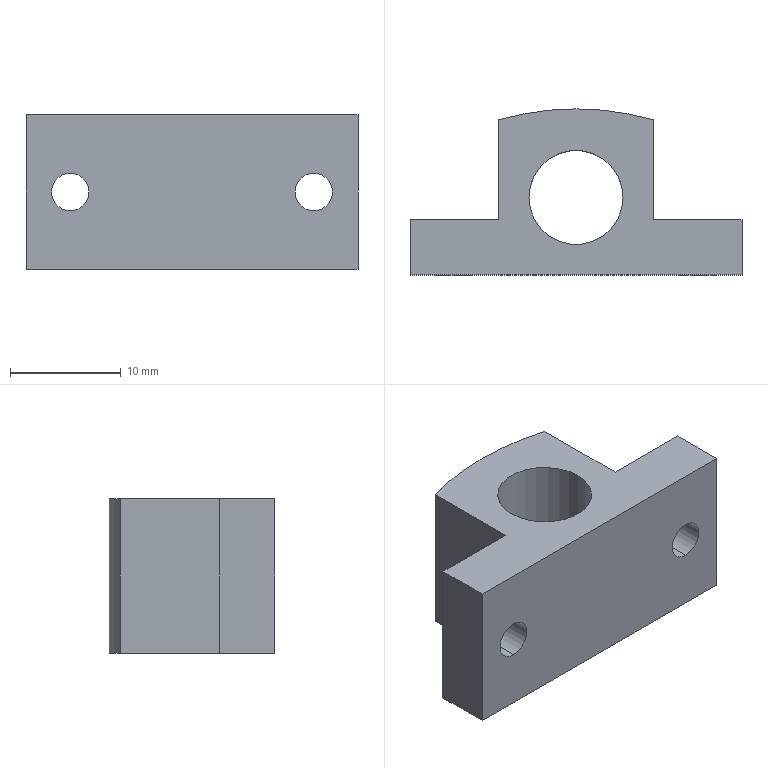Part | SolidWorks | features Extrusion 1, HoleWzd 1, ICE 1 | 1 solid | 20 faces | box 30 x 15 x 14 mm | volume 3079 mm3 | plane 9 | cylinder 7 | cone 4 | commonest cylinder face diameters 3.4 x4 8.5 x2 50 x1
STEP:
#1=CARTESIAN_POINT('',(-4.25,7.,-7.));
#2=VERTEX_POINT('',#1);
#3=CARTESIAN_POINT('',(4.25,7.,-7.));
#4=VERTEX_POINT('',#3);
#5=CARTESIAN_POINT('',(0.,7.,-7.));
#6=DIRECTION('',(0.,0.,1.));
#7=DIRECTION('',(1.,0.,0.));
#8=AXIS2_PLACEMENT_3D('',#5,#6,#7);
#9=CIRCLE('',#8,4.25);
#10=EDGE_CURVE('',#2,#4,#9,.T.);
#11=ORIENTED_EDGE('',*,*,#10,.F.);
#12=CARTESIAN_POINT('',(-4.25,7.,7.));
#13=VERTEX_POINT('',#12);
#14=CARTESIAN_POINT('',(-4.25,7.,-7.));
#15=DIRECTION('',(0.,0.,1.));
#16=VECTOR('',#15,1000.);
#17=LINE('',#14,#16);
#18=EDGE_CURVE('',#2,#13,#17,.T.);
#19=ORIENTED_EDGE('',*,*,#18,.T.);
#20=CARTESIAN_POINT('',(4.25,7.,7.));
#21=VERTEX_POINT('',#20);
#22=CARTESIAN_POINT('',(0.,7.,7.));
#23=DIRECTION('',(0.,0.,1.));
#24=DIRECTION('',(1.,0.,0.));
#25=AXIS2_PLACEMENT_3D('',#22,#23,#24);
#26=CIRCLE('',#25,4.25);
#27=EDGE_CURVE('',#13,#21,#26,.T.);
#28=ORIENTED_EDGE('',*,*,#27,.T.);
#29=CARTESIAN_POINT('',(4.25,7.,-7.));
#30=DIRECTION('',(0.,0.,1.));
#31=VECTOR('',#30,1000.);
#32=LINE('',#29,#31);
#33=EDGE_CURVE('',#4,#21,#32,.T.);
#34=ORIENTED_EDGE('',*,*,#33,.F.);
#35=EDGE_LOOP('',(#11,#19,#28,#34));
#36=FACE_OUTER_BOUND('',#35,.T.);
#37=CARTESIAN_POINT('',(0.,7.,-7.));
#38=DIRECTION('',(0.,0.,1.));
#39=DIRECTION('',(1.,0.,0.));
#40=AXIS2_PLACEMENT_3D('',#37,#38,#39);
#41=CYLINDRICAL_SURFACE('',#40,4.25);
#42=ADVANCED_FACE('',(#36),#41,.F.);
#43=CARTESIAN_POINT('',(-11.,3.5,-1.7));
#44=VERTEX_POINT('',#43);
#45=CARTESIAN_POINT('',(-11.,3.5,1.7));
#46=VERTEX_POINT('',#45);
#47=CARTESIAN_POINT('',(-11.,3.5,0.));
#48=DIRECTION('',(0.,1.,0.));
#49=DIRECTION('',(0.,0.,1.));
#50=AXIS2_PLACEMENT_3D('',#47,#48,#49);
#51=CIRCLE('',#50,1.7);
#52=EDGE_CURVE('',#44,#46,#51,.T.);
#53=ORIENTED_EDGE('',*,*,#52,.F.);
#54=CARTESIAN_POINT('',(-11.,5.,-3.2));
#55=VERTEX_POINT('',#54);
#56=CARTESIAN_POINT('',(-11.,5.,-3.2));
#57=DIRECTION('',(0.,0.7071,-0.7071));
#58=VECTOR('',#57,1000.);
#59=LINE('',#56,#58);
#60=EDGE_CURVE('',#44,#55,#59,.T.);
#61=ORIENTED_EDGE('',*,*,#60,.T.);
#62=CARTESIAN_POINT('',(-11.,5.,3.2));
#63=VERTEX_POINT('',#62);
#64=CARTESIAN_POINT('',(-11.,5.,0.));
#65=DIRECTION('',(0.,1.,0.));
#66=DIRECTION('',(0.,0.,1.));
#67=AXIS2_PLACEMENT_3D('',#64,#65,#66);
#68=CIRCLE('',#67,3.2);
#69=EDGE_CURVE('',#55,#63,#68,.T.);
#70=ORIENTED_EDGE('',*,*,#69,.T.);
#71=CARTESIAN_POINT('',(-11.,5.,3.2));
#72=DIRECTION('',(0.,0.7071,0.7071));
#73=VECTOR('',#72,1000.);
#74=LINE('',#71,#73);
#75=EDGE_CURVE('',#46,#63,#74,.T.);
#76=ORIENTED_EDGE('',*,*,#75,.F.);
#77=EDGE_LOOP('',(#53,#61,#70,#76));
#78=FACE_OUTER_BOUND('',#77,.T.);
#79=CARTESIAN_POINT('',(-11.,5.,0.));
#80=DIRECTION('',(0.,1.,0.));
#81=DIRECTION('',(0.,0.,1.));
#82=AXIS2_PLACEMENT_3D('',#79,#80,#81);
#83=CONICAL_SURFACE('',#82,3.2,0.7854);
#84=ADVANCED_FACE('',(#78),#83,.F.);
#85=CARTESIAN_POINT('',(-11.,0.,-1.7));
#86=VERTEX_POINT('',#85);
#87=CARTESIAN_POINT('',(-11.,0.,1.7));
#88=VERTEX_POINT('',#87);
#89=CARTESIAN_POINT('',(-11.,0.,0.));
#90=DIRECTION('',(0.,1.,0.));
#91=DIRECTION('',(0.,0.,1.));
#92=AXIS2_PLACEMENT_3D('',#89,#90,#91);
#93=CIRCLE('',#92,1.7);
#94=EDGE_CURVE('',#86,#88,#93,.T.);
#95=ORIENTED_EDGE('',*,*,#94,.F.);
#96=CARTESIAN_POINT('',(-11.,5.,-1.7));
#97=DIRECTION('',(0.,1.,0.));
#98=VECTOR('',#97,1000.);
#99=LINE('',#96,#98);
#100=EDGE_CURVE('',#86,#44,#99,.T.);
#101=ORIENTED_EDGE('',*,*,#100,.T.);
#102=ORIENTED_EDGE('',*,*,#52,.T.);
#103=CARTESIAN_POINT('',(-11.,5.,1.7));
#104=DIRECTION('',(0.,1.,0.));
#105=VECTOR('',#104,1000.);
#106=LINE('',#103,#105);
#107=EDGE_CURVE('',#88,#46,#106,.T.);
#108=ORIENTED_EDGE('',*,*,#107,.F.);
#109=EDGE_LOOP('',(#95,#101,#102,#108));
#110=FACE_OUTER_BOUND('',#109,.T.);
#111=CARTESIAN_POINT('',(-11.,5.,0.));
#112=DIRECTION('',(0.,1.,0.));
#113=DIRECTION('',(0.,0.,1.));
#114=AXIS2_PLACEMENT_3D('',#111,#112,#113);
#115=CYLINDRICAL_SURFACE('',#114,1.7);
#116=ADVANCED_FACE('',(#110),#115,.F.);
#117=CARTESIAN_POINT('',(11.,3.5,-1.7));
#118=VERTEX_POINT('',#117);
#119=CARTESIAN_POINT('',(11.,3.5,1.7));
#120=VERTEX_POINT('',#119);
#121=CARTESIAN_POINT('',(11.,3.5,0.));
#122=DIRECTION('',(0.,1.,0.));
#123=DIRECTION('',(0.,0.,1.));
#124=AXIS2_PLACEMENT_3D('',#121,#122,#123);
#125=CIRCLE('',#124,1.7);
#126=EDGE_CURVE('',#118,#120,#125,.T.);
#127=ORIENTED_EDGE('',*,*,#126,.F.);
#128=CARTESIAN_POINT('',(11.,5.,-3.2));
#129=VERTEX_POINT('',#128);
#130=CARTESIAN_POINT('',(11.,5.,-3.2));
#131=DIRECTION('',(0.,0.7071,-0.7071));
#132=VECTOR('',#131,1000.);
#133=LINE('',#130,#132);
#134=EDGE_CURVE('',#118,#129,#133,.T.);
#135=ORIENTED_EDGE('',*,*,#134,.T.);
#136=CARTESIAN_POINT('',(11.,5.,3.2));
#137=VERTEX_POINT('',#136);
#138=CARTESIAN_POINT('',(11.,5.,0.));
#139=DIRECTION('',(0.,1.,0.));
#140=DIRECTION('',(0.,0.,1.));
#141=AXIS2_PLACEMENT_3D('',#138,#139,#140);
#142=CIRCLE('',#141,3.2);
#143=EDGE_CURVE('',#129,#137,#142,.T.);
#144=ORIENTED_EDGE('',*,*,#143,.T.);
#145=CARTESIAN_POINT('',(11.,5.,3.2));
#146=DIRECTION('',(0.,0.7071,0.7071));
#147=VECTOR('',#146,1000.);
#148=LINE('',#145,#147);
#149=EDGE_CURVE('',#120,#137,#148,.T.);
#150=ORIENTED_EDGE('',*,*,#149,.F.);
#151=EDGE_LOOP('',(#127,#135,#144,#150));
#152=FACE_OUTER_BOUND('',#151,.T.);
#153=CARTESIAN_POINT('',(11.,5.,0.));
#154=DIRECTION('',(0.,1.,0.));
#155=DIRECTION('',(0.,0.,1.));
#156=AXIS2_PLACEMENT_3D('',#153,#154,#155);
#157=CONICAL_SURFACE('',#156,3.2,0.7854);
#158=ADVANCED_FACE('',(#152),#157,.F.);
#159=CARTESIAN_POINT('',(11.,0.,-1.7));
#160=VERTEX_POINT('',#159);
#161=CARTESIAN_POINT('',(11.,0.,1.7));
#162=VERTEX_POINT('',#161);
#163=CARTESIAN_POINT('',(11.,0.,0.));
#164=DIRECTION('',(0.,1.,0.));
#165=DIRECTION('',(0.,0.,1.));
#166=AXIS2_PLACEMENT_3D('',#163,#164,#165);
#167=CIRCLE('',#166,1.7);
#168=EDGE_CURVE('',#160,#162,#167,.T.);
#169=ORIENTED_EDGE('',*,*,#168,.F.);
#170=CARTESIAN_POINT('',(11.,5.,-1.7));
#171=DIRECTION('',(0.,1.,0.));
#172=VECTOR('',#171,1000.);
#173=LINE('',#170,#172);
#174=EDGE_CURVE('',#160,#118,#173,.T.);
#175=ORIENTED_EDGE('',*,*,#174,.T.);
#176=ORIENTED_EDGE('',*,*,#126,.T.);
#177=CARTESIAN_POINT('',(11.,5.,1.7));
#178=DIRECTION('',(0.,1.,0.));
#179=VECTOR('',#178,1000.);
#180=LINE('',#177,#179);
#181=EDGE_CURVE('',#162,#120,#180,.T.);
#182=ORIENTED_EDGE('',*,*,#181,.F.);
#183=EDGE_LOOP('',(#169,#175,#176,#182));
#184=FACE_OUTER_BOUND('',#183,.T.);
#185=CARTESIAN_POINT('',(11.,5.,0.));
#186=DIRECTION('',(0.,1.,0.));
#187=DIRECTION('',(0.,0.,1.));
#188=AXIS2_PLACEMENT_3D('',#185,#186,#187);
#189=CYLINDRICAL_SURFACE('',#188,1.7);
#190=ADVANCED_FACE('',(#184),#189,.F.);
#191=CARTESIAN_POINT('',(15.,0.,-7.));
#192=VERTEX_POINT('',#191);
#193=CARTESIAN_POINT('',(15.,5.,-7.));
#194=VERTEX_POINT('',#193);
#195=CARTESIAN_POINT('',(15.,5.,-7.));
#196=DIRECTION('',(0.,1.,0.));
#197=VECTOR('',#196,1000.);
#198=LINE('',#195,#197);
#199=EDGE_CURVE('',#192,#194,#198,.T.);
#200=ORIENTED_EDGE('',*,*,#199,.T.);
#201=CARTESIAN_POINT('',(15.,5.,7.));
#202=VERTEX_POINT('',#201);
#203=CARTESIAN_POINT('',(15.,5.,7.));
#204=DIRECTION('',(0.,0.,-1.));
#205=VECTOR('',#204,1000.);
#206=LINE('',#203,#205);
#207=EDGE_CURVE('',#202,#194,#206,.T.);
#208=ORIENTED_EDGE('',*,*,#207,.F.);
#209=CARTESIAN_POINT('',(15.,0.,7.));
#210=VERTEX_POINT('',#209);
#211=CARTESIAN_POINT('',(15.,5.,7.));
#212=DIRECTION('',(0.,1.,0.));
#213=VECTOR('',#212,1000.);
#214=LINE('',#211,#213);
#215=EDGE_CURVE('',#210,#202,#214,.T.);
#216=ORIENTED_EDGE('',*,*,#215,.F.);
#217=CARTESIAN_POINT('',(15.,0.,7.));
#218=DIRECTION('',(0.,0.,-1.));
#219=VECTOR('',#218,1000.);
#220=LINE('',#217,#219);
#221=EDGE_CURVE('',#210,#192,#220,.T.);
#222=ORIENTED_EDGE('',*,*,#221,.T.);
#223=EDGE_LOOP('',(#200,#208,#216,#222));
#224=FACE_OUTER_BOUND('',#223,.T.);
#225=CARTESIAN_POINT('',(15.,5.,7.));
#226=DIRECTION('',(-1.,0.,0.));
#227=DIRECTION('',(0.,-1.,0.));
#228=AXIS2_PLACEMENT_3D('',#225,#226,#227);
#229=PLANE('',#228);
#230=ADVANCED_FACE('',(#224),#229,.F.);
#231=CARTESIAN_POINT('',(11.,5.,0.));
#232=DIRECTION('',(0.,1.,0.));
#233=DIRECTION('',(0.,0.,1.));
#234=AXIS2_PLACEMENT_3D('',#231,#232,#233);
#235=CIRCLE('',#234,3.2);
#236=EDGE_CURVE('',#137,#129,#235,.T.);
#237=ORIENTED_EDGE('',*,*,#236,.F.);
#238=ORIENTED_EDGE('',*,*,#143,.F.);
#239=EDGE_LOOP('',(#237,#238));
#240=FACE_BOUND('',#239,.T.);
#241=CARTESIAN_POINT('',(7.,5.,-7.));
#242=VERTEX_POINT('',#241);
#243=CARTESIAN_POINT('',(15.,5.,-7.));
#244=DIRECTION('',(-1.,0.,0.));
#245=VECTOR('',#244,1000.);
#246=LINE('',#243,#245);
#247=EDGE_CURVE('',#194,#242,#246,.T.);
#248=ORIENTED_EDGE('',*,*,#247,.T.);
#249=CARTESIAN_POINT('',(7.,5.,7.));
#250=VERTEX_POINT('',#249);
#251=CARTESIAN_POINT('',(7.,5.,7.));
#252=DIRECTION('',(0.,0.,-1.));
#253=VECTOR('',#252,1000.);
#254=LINE('',#251,#253);
#255=EDGE_CURVE('',#250,#242,#254,.T.);
#256=ORIENTED_EDGE('',*,*,#255,.F.);
#257=CARTESIAN_POINT('',(15.,5.,7.));
#258=DIRECTION('',(-1.,0.,0.));
#259=VECTOR('',#258,1000.);
#260=LINE('',#257,#259);
#261=EDGE_CURVE('',#202,#250,#260,.T.);
#262=ORIENTED_EDGE('',*,*,#261,.F.);
#263=ORIENTED_EDGE('',*,*,#207,.T.);
#264=EDGE_LOOP('',(#248,#256,#262,#263));
#265=FACE_OUTER_BOUND('',#264,.T.);
#266=CARTESIAN_POINT('',(15.,5.,7.));
#267=DIRECTION('',(0.,-1.,0.));
#268=DIRECTION('',(1.,0.,0.));
#269=AXIS2_PLACEMENT_3D('',#266,#267,#268);
#270=PLANE('',#269);
#271=ADVANCED_FACE('',(#240,#265),#270,.F.);
#272=CARTESIAN_POINT('',(7.,14.,-7.));
#273=VERTEX_POINT('',#272);
#274=CARTESIAN_POINT('',(7.,5.,-7.));
#275=DIRECTION('',(0.,1.,0.));
#276=VECTOR('',#275,1000.);
#277=LINE('',#274,#276);
#278=EDGE_CURVE('',#242,#273,#277,.T.);
#279=ORIENTED_EDGE('',*,*,#278,.T.);
#280=CARTESIAN_POINT('',(7.,14.,7.));
#281=VERTEX_POINT('',#280);
#282=CARTESIAN_POINT('',(7.,14.,7.));
#283=DIRECTION('',(0.,0.,-1.));
#284=VECTOR('',#283,1000.);
#285=LINE('',#282,#284);
#286=EDGE_CURVE('',#281,#273,#285,.T.);
#287=ORIENTED_EDGE('',*,*,#286,.F.);
#288=CARTESIAN_POINT('',(7.,5.,7.));
#289=DIRECTION('',(0.,1.,0.));
#290=VECTOR('',#289,1000.);
#291=LINE('',#288,#290);
#292=EDGE_CURVE('',#250,#281,#291,.T.);
#293=ORIENTED_EDGE('',*,*,#292,.F.);
#294=ORIENTED_EDGE('',*,*,#255,.T.);
#295=EDGE_LOOP('',(#279,#287,#293,#294));
#296=FACE_OUTER_BOUND('',#295,.T.);
#297=CARTESIAN_POINT('',(7.,5.,7.));
#298=DIRECTION('',(-1.,0.,0.));
#299=DIRECTION('',(0.,-1.,0.));
#300=AXIS2_PLACEMENT_3D('',#297,#298,#299);
#301=PLANE('',#300);
#302=ADVANCED_FACE('',(#296),#301,.F.);
#303=CARTESIAN_POINT('',(-7.,14.,-7.));
#304=VERTEX_POINT('',#303);
#305=CARTESIAN_POINT('',(0.,-10.,-7.));
#306=DIRECTION('',(0.,0.,1.));
#307=DIRECTION('',(-1.,0.,0.));
#308=AXIS2_PLACEMENT_3D('',#305,#306,#307);
#309=CIRCLE('',#308,25.);
#310=EDGE_CURVE('',#273,#304,#309,.T.);
#311=ORIENTED_EDGE('',*,*,#310,.T.);
#312=CARTESIAN_POINT('',(-7.,14.,7.));
#313=VERTEX_POINT('',#312);
#314=CARTESIAN_POINT('',(-7.,14.,7.));
#315=DIRECTION('',(0.,0.,-1.));
#316=VECTOR('',#315,1000.);
#317=LINE('',#314,#316);
#318=EDGE_CURVE('',#313,#304,#317,.T.);
#319=ORIENTED_EDGE('',*,*,#318,.F.);
#320=CARTESIAN_POINT('',(0.,-10.,7.));
#321=DIRECTION('',(0.,0.,1.));
#322=DIRECTION('',(-1.,0.,0.));
#323=AXIS2_PLACEMENT_3D('',#320,#321,#322);
#324=CIRCLE('',#323,25.);
#325=EDGE_CURVE('',#281,#313,#324,.T.);
#326=ORIENTED_EDGE('',*,*,#325,.F.);
#327=ORIENTED_EDGE('',*,*,#286,.T.);
#328=EDGE_LOOP('',(#311,#319,#326,#327));
#329=FACE_OUTER_BOUND('',#328,.T.);
#330=CARTESIAN_POINT('',(0.,-10.,7.));
#331=DIRECTION('',(0.,0.,-1.));
#332=DIRECTION('',(-1.,0.,0.));
#333=AXIS2_PLACEMENT_3D('',#330,#331,#332);
#334=CYLINDRICAL_SURFACE('',#333,25.);
#335=ADVANCED_FACE('',(#329),#334,.T.);
#336=CARTESIAN_POINT('',(-7.,5.,-7.));
#337=VERTEX_POINT('',#336);
#338=CARTESIAN_POINT('',(-7.,5.,-7.));
#339=DIRECTION('',(0.,-1.,0.));
#340=VECTOR('',#339,1000.);
#341=LINE('',#338,#340);
#342=EDGE_CURVE('',#304,#337,#341,.T.);
#343=ORIENTED_EDGE('',*,*,#342,.T.);
#344=CARTESIAN_POINT('',(-7.,5.,7.));
#345=VERTEX_POINT('',#344);
#346=CARTESIAN_POINT('',(-7.,5.,7.));
#347=DIRECTION('',(0.,0.,-1.));
#348=VECTOR('',#347,1000.);
#349=LINE('',#346,#348);
#350=EDGE_CURVE('',#345,#337,#349,.T.);
#351=ORIENTED_EDGE('',*,*,#350,.F.);
#352=CARTESIAN_POINT('',(-7.,5.,7.));
#353=DIRECTION('',(0.,-1.,0.));
#354=VECTOR('',#353,1000.);
#355=LINE('',#352,#354);
#356=EDGE_CURVE('',#313,#345,#355,.T.);
#357=ORIENTED_EDGE('',*,*,#356,.F.);
#358=ORIENTED_EDGE('',*,*,#318,.T.);
#359=EDGE_LOOP('',(#343,#351,#357,#358));
#360=FACE_OUTER_BOUND('',#359,.T.);
#361=CARTESIAN_POINT('',(-7.,5.,7.));
#362=DIRECTION('',(1.,0.,0.));
#363=DIRECTION('',(0.,0.,-1.));
#364=AXIS2_PLACEMENT_3D('',#361,#362,#363);
#365=PLANE('',#364);
#366=ADVANCED_FACE('',(#360),#365,.F.);
#367=CARTESIAN_POINT('',(-11.,5.,0.));
#368=DIRECTION('',(0.,1.,0.));
#369=DIRECTION('',(0.,0.,1.));
#370=AXIS2_PLACEMENT_3D('',#367,#368,#369);
#371=CIRCLE('',#370,3.2);
#372=EDGE_CURVE('',#63,#55,#371,.T.);
#373=ORIENTED_EDGE('',*,*,#372,.F.);
#374=ORIENTED_EDGE('',*,*,#69,.F.);
#375=EDGE_LOOP('',(#373,#374));
#376=FACE_BOUND('',#375,.T.);
#377=CARTESIAN_POINT('',(-15.,5.,-7.));
#378=VERTEX_POINT('',#377);
#379=CARTESIAN_POINT('',(-15.,5.,-7.));
#380=DIRECTION('',(-1.,0.,0.));
#381=VECTOR('',#380,1000.);
#382=LINE('',#379,#381);
#383=EDGE_CURVE('',#337,#378,#382,.T.);
#384=ORIENTED_EDGE('',*,*,#383,.T.);
#385=CARTESIAN_POINT('',(-15.,5.,7.));
#386=VERTEX_POINT('',#385);
#387=CARTESIAN_POINT('',(-15.,5.,7.));
#388=DIRECTION('',(0.,0.,-1.));
#389=VECTOR('',#388,1000.);
#390=LINE('',#387,#389);
#391=EDGE_CURVE('',#386,#378,#390,.T.);
#392=ORIENTED_EDGE('',*,*,#391,.F.);
#393=CARTESIAN_POINT('',(-15.,5.,7.));
#394=DIRECTION('',(-1.,0.,0.));
#395=VECTOR('',#394,1000.);
#396=LINE('',#393,#395);
#397=EDGE_CURVE('',#345,#386,#396,.T.);
#398=ORIENTED_EDGE('',*,*,#397,.F.);
#399=ORIENTED_EDGE('',*,*,#350,.T.);
#400=EDGE_LOOP('',(#384,#392,#398,#399));
#401=FACE_OUTER_BOUND('',#400,.T.);
#402=CARTESIAN_POINT('',(-15.,5.,7.));
#403=DIRECTION('',(0.,-1.,0.));
#404=DIRECTION('',(0.,0.,-1.));
#405=AXIS2_PLACEMENT_3D('',#402,#403,#404);
#406=PLANE('',#405);
#407=ADVANCED_FACE('',(#376,#401),#406,.F.);
#408=CARTESIAN_POINT('',(-15.,0.,-7.));
#409=VERTEX_POINT('',#408);
#410=CARTESIAN_POINT('',(-15.,5.,-7.));
#411=DIRECTION('',(0.,-1.,0.));
#412=VECTOR('',#411,1000.);
#413=LINE('',#410,#412);
#414=EDGE_CURVE('',#378,#409,#413,.T.);
#415=ORIENTED_EDGE('',*,*,#414,.T.);
#416=CARTESIAN_POINT('',(-15.,0.,7.));
#417=VERTEX_POINT('',#416);
#418=CARTESIAN_POINT('',(-15.,0.,7.));
#419=DIRECTION('',(0.,0.,-1.));
#420=VECTOR('',#419,1000.);
#421=LINE('',#418,#420);
#422=EDGE_CURVE('',#417,#409,#421,.T.);
#423=ORIENTED_EDGE('',*,*,#422,.F.);
#424=CARTESIAN_POINT('',(-15.,5.,7.));
#425=DIRECTION('',(0.,-1.,0.));
#426=VECTOR('',#425,1000.);
#427=LINE('',#424,#426);
#428=EDGE_CURVE('',#386,#417,#427,.T.);
#429=ORIENTED_EDGE('',*,*,#428,.F.);
#430=ORIENTED_EDGE('',*,*,#391,.T.);
#431=EDGE_LOOP('',(#415,#423,#429,#430));
#432=FACE_OUTER_BOUND('',#431,.T.);
#433=CARTESIAN_POINT('',(-15.,5.,7.));
#434=DIRECTION('',(1.,0.,0.));
#435=DIRECTION('',(0.,0.,-1.));
#436=AXIS2_PLACEMENT_3D('',#433,#434,#435);
#437=PLANE('',#436);
#438=ADVANCED_FACE('',(#432),#437,.F.);
#439=CARTESIAN_POINT('',(-11.,0.,0.));
#440=DIRECTION('',(0.,1.,0.));
#441=DIRECTION('',(0.,0.,1.));
#442=AXIS2_PLACEMENT_3D('',#439,#440,#441);
#443=CIRCLE('',#442,1.7);
#444=EDGE_CURVE('',#88,#86,#443,.T.);
#445=ORIENTED_EDGE('',*,*,#444,.T.);
#446=ORIENTED_EDGE('',*,*,#94,.T.);
#447=EDGE_LOOP('',(#445,#446));
#448=FACE_BOUND('',#447,.T.);
#449=CARTESIAN_POINT('',(11.,0.,0.));
#450=DIRECTION('',(0.,1.,0.));
#451=DIRECTION('',(0.,0.,1.));
#452=AXIS2_PLACEMENT_3D('',#449,#450,#451);
#453=CIRCLE('',#452,1.7);
#454=EDGE_CURVE('',#162,#160,#453,.T.);
#455=ORIENTED_EDGE('',*,*,#454,.T.);
#456=ORIENTED_EDGE('',*,*,#168,.T.);
#457=EDGE_LOOP('',(#455,#456));
#458=FACE_BOUND('',#457,.T.);
#459=CARTESIAN_POINT('',(-15.,0.,-7.));
#460=DIRECTION('',(1.,0.,0.));
#461=VECTOR('',#460,1000.);
#462=LINE('',#459,#461);
#463=EDGE_CURVE('',#409,#192,#462,.T.);
#464=ORIENTED_EDGE('',*,*,#463,.T.);
#465=ORIENTED_EDGE('',*,*,#221,.F.);
#466=CARTESIAN_POINT('',(-15.,0.,7.));
#467=DIRECTION('',(1.,0.,0.));
#468=VECTOR('',#467,1000.);
#469=LINE('',#466,#468);
#470=EDGE_CURVE('',#417,#210,#469,.T.);
#471=ORIENTED_EDGE('',*,*,#470,.F.);
#472=ORIENTED_EDGE('',*,*,#422,.T.);
#473=EDGE_LOOP('',(#464,#465,#471,#472));
#474=FACE_OUTER_BOUND('',#473,.T.);
#475=CARTESIAN_POINT('',(-15.,0.,7.));
#476=DIRECTION('',(0.,1.,0.));
#477=DIRECTION('',(-1.,0.,0.));
#478=AXIS2_PLACEMENT_3D('',#475,#476,#477);
#479=PLANE('',#478);
#480=ADVANCED_FACE('',(#448,#458,#474),#479,.F.);
#481=CARTESIAN_POINT('',(0.,7.,7.));
#482=DIRECTION('',(0.,0.,1.));
#483=DIRECTION('',(1.,0.,0.));
#484=AXIS2_PLACEMENT_3D('',#481,#482,#483);
#485=CIRCLE('',#484,4.25);
#486=EDGE_CURVE('',#21,#13,#485,.T.);
#487=ORIENTED_EDGE('',*,*,#486,.F.);
#488=ORIENTED_EDGE('',*,*,#27,.F.);
#489=EDGE_LOOP('',(#487,#488));
#490=FACE_BOUND('',#489,.T.);
#491=ORIENTED_EDGE('',*,*,#215,.T.);
#492=ORIENTED_EDGE('',*,*,#261,.T.);
#493=ORIENTED_EDGE('',*,*,#292,.T.);
#494=ORIENTED_EDGE('',*,*,#325,.T.);
#495=ORIENTED_EDGE('',*,*,#356,.T.);
#496=ORIENTED_EDGE('',*,*,#397,.T.);
#497=ORIENTED_EDGE('',*,*,#428,.T.);
#498=ORIENTED_EDGE('',*,*,#470,.T.);
#499=EDGE_LOOP('',(#491,#492,#493,#494,#495,#496,#497,#498));
#500=FACE_OUTER_BOUND('',#499,.T.);
#501=CARTESIAN_POINT('',(0.,-10.,7.));
#502=DIRECTION('',(0.,0.,-1.));
#503=DIRECTION('',(-1.,0.,0.));
#504=AXIS2_PLACEMENT_3D('',#501,#502,#503);
#505=PLANE('',#504);
#506=ADVANCED_FACE('',(#490,#500),#505,.F.);
#507=CARTESIAN_POINT('',(0.,7.,-7.));
#508=DIRECTION('',(0.,0.,1.));
#509=DIRECTION('',(1.,0.,0.));
#510=AXIS2_PLACEMENT_3D('',#507,#508,#509);
#511=CIRCLE('',#510,4.25);
#512=EDGE_CURVE('',#4,#2,#511,.T.);
#513=ORIENTED_EDGE('',*,*,#512,.T.);
#514=ORIENTED_EDGE('',*,*,#10,.T.);
#515=EDGE_LOOP('',(#513,#514));
#516=FACE_BOUND('',#515,.T.);
#517=ORIENTED_EDGE('',*,*,#199,.F.);
#518=ORIENTED_EDGE('',*,*,#463,.F.);
#519=ORIENTED_EDGE('',*,*,#414,.F.);
#520=ORIENTED_EDGE('',*,*,#383,.F.);
#521=ORIENTED_EDGE('',*,*,#342,.F.);
#522=ORIENTED_EDGE('',*,*,#310,.F.);
#523=ORIENTED_EDGE('',*,*,#278,.F.);
#524=ORIENTED_EDGE('',*,*,#247,.F.);
#525=EDGE_LOOP('',(#517,#518,#519,#520,#521,#522,#523,#524));
#526=FACE_OUTER_BOUND('',#525,.T.);
#527=CARTESIAN_POINT('',(0.,-10.,-7.));
#528=DIRECTION('',(0.,0.,-1.));
#529=DIRECTION('',(-1.,0.,0.));
#530=AXIS2_PLACEMENT_3D('',#527,#528,#529);
#531=PLANE('',#530);
#532=ADVANCED_FACE('',(#516,#526),#531,.T.);
#533=ORIENTED_EDGE('',*,*,#174,.F.);
#534=ORIENTED_EDGE('',*,*,#454,.F.);
#535=ORIENTED_EDGE('',*,*,#181,.T.);
#536=CARTESIAN_POINT('',(11.,3.5,0.));
#537=DIRECTION('',(0.,1.,0.));
#538=DIRECTION('',(0.,0.,1.));
#539=AXIS2_PLACEMENT_3D('',#536,#537,#538);
#540=CIRCLE('',#539,1.7);
#541=EDGE_CURVE('',#120,#118,#540,.T.);
#542=ORIENTED_EDGE('',*,*,#541,.T.);
#543=EDGE_LOOP('',(#533,#534,#535,#542));
#544=FACE_OUTER_BOUND('',#543,.T.);
#545=CARTESIAN_POINT('',(11.,5.,0.));
#546=DIRECTION('',(0.,1.,0.));
#547=DIRECTION('',(0.,0.,1.));
#548=AXIS2_PLACEMENT_3D('',#545,#546,#547);
#549=CYLINDRICAL_SURFACE('',#548,1.7);
#550=ADVANCED_FACE('',(#544),#549,.F.);
#551=ORIENTED_EDGE('',*,*,#134,.F.);
#552=ORIENTED_EDGE('',*,*,#541,.F.);
#553=ORIENTED_EDGE('',*,*,#149,.T.);
#554=ORIENTED_EDGE('',*,*,#236,.T.);
#555=EDGE_LOOP('',(#551,#552,#553,#554));
#556=FACE_OUTER_BOUND('',#555,.T.);
#557=CARTESIAN_POINT('',(11.,5.,0.));
#558=DIRECTION('',(0.,1.,0.));
#559=DIRECTION('',(0.,0.,1.));
#560=AXIS2_PLACEMENT_3D('',#557,#558,#559);
#561=CONICAL_SURFACE('',#560,3.2,0.7854);
#562=ADVANCED_FACE('',(#556),#561,.F.);
#563=ORIENTED_EDGE('',*,*,#100,.F.);
#564=ORIENTED_EDGE('',*,*,#444,.F.);
#565=ORIENTED_EDGE('',*,*,#107,.T.);
#566=CARTESIAN_POINT('',(-11.,3.5,0.));
#567=DIRECTION('',(0.,1.,0.));
#568=DIRECTION('',(0.,0.,1.));
#569=AXIS2_PLACEMENT_3D('',#566,#567,#568);
#570=CIRCLE('',#569,1.7);
#571=EDGE_CURVE('',#46,#44,#570,.T.);
#572=ORIENTED_EDGE('',*,*,#571,.T.);
#573=EDGE_LOOP('',(#563,#564,#565,#572));
#574=FACE_OUTER_BOUND('',#573,.T.);
#575=CARTESIAN_POINT('',(-11.,5.,0.));
#576=DIRECTION('',(0.,1.,0.));
#577=DIRECTION('',(0.,0.,1.));
#578=AXIS2_PLACEMENT_3D('',#575,#576,#577);
#579=CYLINDRICAL_SURFACE('',#578,1.7);
#580=ADVANCED_FACE('',(#574),#579,.F.);
#581=ORIENTED_EDGE('',*,*,#60,.F.);
#582=ORIENTED_EDGE('',*,*,#571,.F.);
#583=ORIENTED_EDGE('',*,*,#75,.T.);
#584=ORIENTED_EDGE('',*,*,#372,.T.);
#585=EDGE_LOOP('',(#581,#582,#583,#584));
#586=FACE_OUTER_BOUND('',#585,.T.);
#587=CARTESIAN_POINT('',(-11.,5.,0.));
#588=DIRECTION('',(0.,1.,0.));
#589=DIRECTION('',(0.,0.,1.));
#590=AXIS2_PLACEMENT_3D('',#587,#588,#589);
#591=CONICAL_SURFACE('',#590,3.2,0.7854);
#592=ADVANCED_FACE('',(#586),#591,.F.);
#593=ORIENTED_EDGE('',*,*,#18,.F.);
#594=ORIENTED_EDGE('',*,*,#512,.F.);
#595=ORIENTED_EDGE('',*,*,#33,.T.);
#596=ORIENTED_EDGE('',*,*,#486,.T.);
#597=EDGE_LOOP('',(#593,#594,#595,#596));
#598=FACE_OUTER_BOUND('',#597,.T.);
#599=CARTESIAN_POINT('',(0.,7.,-7.));
#600=DIRECTION('',(0.,0.,1.));
#601=DIRECTION('',(1.,0.,0.));
#602=AXIS2_PLACEMENT_3D('',#599,#600,#601);
#603=CYLINDRICAL_SURFACE('',#602,4.25);
#604=ADVANCED_FACE('',(#598),#603,.F.);
#605=CLOSED_SHELL('',(#42,#84,#116,#158,#190,#230,#271,#302,#335,#366,#407,#438,#480,#506,#532,#550,#562,#580,#592,#604));
#606=MANIFOLD_SOLID_BREP('',#605);
#607=CARTESIAN_POINT('',(0.,0.,0.));
#608=DIRECTION('',(0.,0.,1.));
#609=DIRECTION('',(1.,0.,0.));
#610=AXIS2_PLACEMENT_3D('',#607,#608,#609);
#611=(LENGTH_UNIT()NAMED_UNIT(*)SI_UNIT(.MILLI.,.METRE.));
#612=UNCERTAINTY_MEASURE_WITH_UNIT(LENGTH_MEASURE(0.00001),#611,'','');
#613=(NAMED_UNIT(*)PLANE_ANGLE_UNIT()SI_UNIT($,.RADIAN.));
#614=(NAMED_UNIT(*)SI_UNIT($,.STERADIAN.)SOLID_ANGLE_UNIT());
#615=(GEOMETRIC_REPRESENTATION_CONTEXT(3)GLOBAL_UNCERTAINTY_ASSIGNED_CONTEXT((#612))GLOBAL_UNIT_ASSIGNED_CONTEXT((#611,#613,#614))REPRESENTATION_CONTEXT('',''));
#616=ADVANCED_BREP_SHAPE_REPRESENTATION('',(#606,#610),#615);